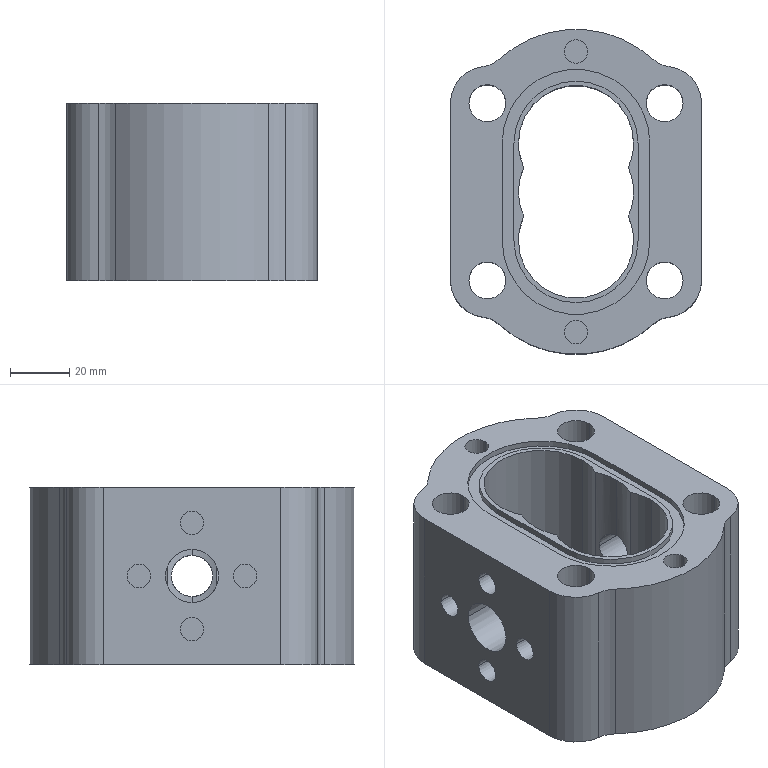Part | SolidWorks | features ICE 7, MirrorPattern 2, Extrusion 1, Fillet 1 | 1 solid | 86 faces | box 85 x 110 x 60 mm | volume 289400 mm3 | cylinder 60 | plane 26 | commonest cylinder face diameters 8 x20 39 x10 12.5 x8 20 x4 25 x4 42 x4